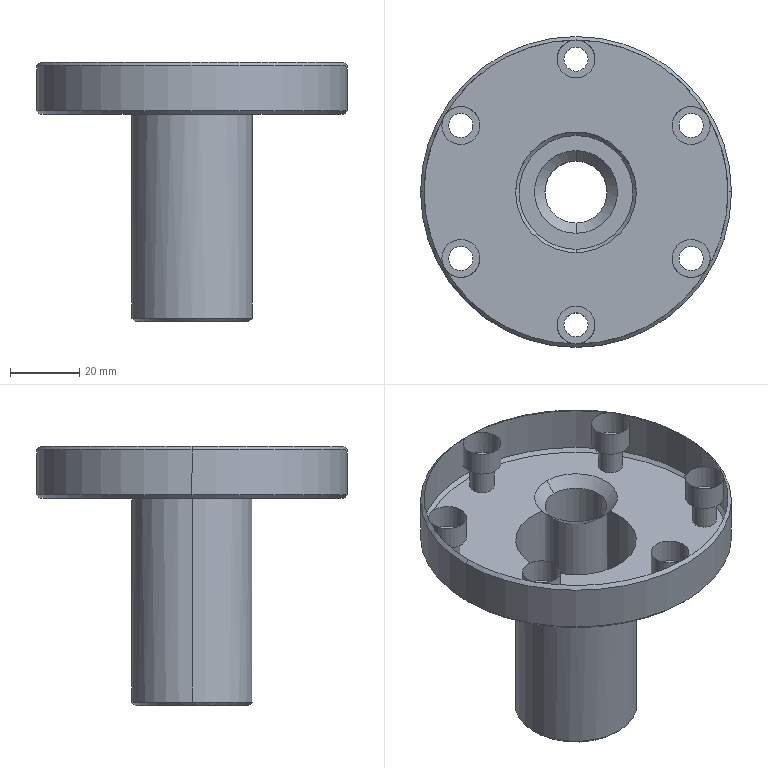Part | STEP file | Tail End Cover | 1 solid | 49 faces | box 90 x 90 x 75 mm | volume 127582 mm3 | cylinder 30 | cone 10 | plane 9 | commonest cylinder face diameters 7 x12 11 x12 18 x2 35 x2 90 x2
STEP:
#1=CARTESIAN_POINT('',(44.,0.,15.));
#2=VERTEX_POINT('',#1);
#3=CARTESIAN_POINT('',(0.,44.,15.));
#4=VERTEX_POINT('',#3);
#5=CARTESIAN_POINT('',(0.,0.,15.));
#6=DIRECTION('',(0.,0.,1.));
#7=DIRECTION('',(-1.,0.,0.));
#8=AXIS2_PLACEMENT_3D('',#5,#6,#7);
#9=CIRCLE('',#8,44.);
#10=EDGE_CURVE('',#2,#4,#9,.T.);
#11=ORIENTED_EDGE('',*,*,#10,.F.);
#12=CARTESIAN_POINT('',(45.,0.,14.));
#13=VERTEX_POINT('',#12);
#14=CARTESIAN_POINT('',(45.,0.,14.));
#15=DIRECTION('',(0.7071,0.,-0.7071));
#16=VECTOR('',#15,1000.);
#17=LINE('',#14,#16);
#18=EDGE_CURVE('',#2,#13,#17,.T.);
#19=ORIENTED_EDGE('',*,*,#18,.T.);
#20=CARTESIAN_POINT('',(-45.,0.,14.));
#21=VERTEX_POINT('',#20);
#22=CARTESIAN_POINT('',(0.,0.,14.));
#23=DIRECTION('',(0.,0.,1.));
#24=DIRECTION('',(-1.,0.,0.));
#25=AXIS2_PLACEMENT_3D('',#22,#23,#24);
#26=CIRCLE('',#25,45.);
#27=EDGE_CURVE('',#13,#21,#26,.T.);
#28=ORIENTED_EDGE('',*,*,#27,.T.);
#29=CARTESIAN_POINT('',(-44.,0.,15.));
#30=VERTEX_POINT('',#29);
#31=CARTESIAN_POINT('',(-45.,0.,14.));
#32=DIRECTION('',(-0.7071,0.,-0.7071));
#33=VECTOR('',#32,1000.);
#34=LINE('',#31,#33);
#35=EDGE_CURVE('',#30,#21,#34,.T.);
#36=ORIENTED_EDGE('',*,*,#35,.F.);
#37=CARTESIAN_POINT('',(-38.105,22.,15.));
#38=VERTEX_POINT('',#37);
#39=CARTESIAN_POINT('',(0.,0.,15.));
#40=DIRECTION('',(0.,0.,1.));
#41=DIRECTION('',(-1.,0.,0.));
#42=AXIS2_PLACEMENT_3D('',#39,#40,#41);
#43=CIRCLE('',#42,44.);
#44=EDGE_CURVE('',#38,#30,#43,.T.);
#45=ORIENTED_EDGE('',*,*,#44,.F.);
#46=CARTESIAN_POINT('',(0.,0.,15.));
#47=DIRECTION('',(0.,0.,1.));
#48=DIRECTION('',(-1.,0.,0.));
#49=AXIS2_PLACEMENT_3D('',#46,#47,#48);
#50=CIRCLE('',#49,44.);
#51=EDGE_CURVE('',#4,#38,#50,.T.);
#52=ORIENTED_EDGE('',*,*,#51,.F.);
#53=EDGE_LOOP('',(#11,#19,#28,#36,#45,#52));
#54=FACE_OUTER_BOUND('',#53,.T.);
#55=CARTESIAN_POINT('',(0.,0.,14.));
#56=DIRECTION('',(0.,0.,-1.));
#57=DIRECTION('',(-1.,0.,0.));
#58=AXIS2_PLACEMENT_3D('',#55,#56,#57);
#59=CONICAL_SURFACE('',#58,45.,0.7854);
#60=ADVANCED_FACE('',(#54),#59,.T.);
#61=CARTESIAN_POINT('',(27.842,-19.25,8.));
#62=VERTEX_POINT('',#61);
#63=CARTESIAN_POINT('',(38.842,-19.25,8.));
#64=VERTEX_POINT('',#63);
#65=CARTESIAN_POINT('',(33.342,-19.25,8.));
#66=DIRECTION('',(0.,0.,1.));
#67=DIRECTION('',(1.,0.,0.));
#68=AXIS2_PLACEMENT_3D('',#65,#66,#67);
#69=CIRCLE('',#68,5.5);
#70=EDGE_CURVE('',#62,#64,#69,.T.);
#71=ORIENTED_EDGE('',*,*,#70,.F.);
#72=CARTESIAN_POINT('',(27.842,-19.25,15.));
#73=VERTEX_POINT('',#72);
#74=CARTESIAN_POINT('',(27.842,-19.25,8.));
#75=DIRECTION('',(0.,0.,1.));
#76=VECTOR('',#75,1000.);
#77=LINE('',#74,#76);
#78=EDGE_CURVE('',#62,#73,#77,.T.);
#79=ORIENTED_EDGE('',*,*,#78,.T.);
#80=CARTESIAN_POINT('',(38.105,-22.,15.));
#81=VERTEX_POINT('',#80);
#82=CARTESIAN_POINT('',(33.342,-19.25,15.));
#83=DIRECTION('',(0.,0.,-1.));
#84=DIRECTION('',(1.,0.,0.));
#85=AXIS2_PLACEMENT_3D('',#82,#83,#84);
#86=CIRCLE('',#85,5.5);
#87=EDGE_CURVE('',#81,#73,#86,.T.);
#88=ORIENTED_EDGE('',*,*,#87,.F.);
#89=CARTESIAN_POINT('',(38.842,-19.25,15.));
#90=VERTEX_POINT('',#89);
#91=CARTESIAN_POINT('',(33.342,-19.25,15.));
#92=DIRECTION('',(0.,0.,-1.));
#93=DIRECTION('',(1.,0.,0.));
#94=AXIS2_PLACEMENT_3D('',#91,#92,#93);
#95=CIRCLE('',#94,5.5);
#96=EDGE_CURVE('',#90,#81,#95,.T.);
#97=ORIENTED_EDGE('',*,*,#96,.F.);
#98=CARTESIAN_POINT('',(38.842,-19.25,8.));
#99=DIRECTION('',(0.,0.,1.));
#100=VECTOR('',#99,1000.);
#101=LINE('',#98,#100);
#102=EDGE_CURVE('',#64,#90,#101,.T.);
#103=ORIENTED_EDGE('',*,*,#102,.F.);
#104=EDGE_LOOP('',(#71,#79,#88,#97,#103));
#105=FACE_OUTER_BOUND('',#104,.T.);
#106=CARTESIAN_POINT('',(33.342,-19.25,8.));
#107=DIRECTION('',(0.,0.,1.));
#108=DIRECTION('',(1.,0.,0.));
#109=AXIS2_PLACEMENT_3D('',#106,#107,#108);
#110=CYLINDRICAL_SURFACE('',#109,5.5);
#111=ADVANCED_FACE('',(#105),#110,.F.);
#112=CARTESIAN_POINT('',(-5.5,-38.5,8.));
#113=VERTEX_POINT('',#112);
#114=CARTESIAN_POINT('',(5.5,-38.5,8.));
#115=VERTEX_POINT('',#114);
#116=CARTESIAN_POINT('',(0.,-38.5,8.));
#117=DIRECTION('',(0.,0.,1.));
#118=DIRECTION('',(1.,0.,0.));
#119=AXIS2_PLACEMENT_3D('',#116,#117,#118);
#120=CIRCLE('',#119,5.5);
#121=EDGE_CURVE('',#113,#115,#120,.T.);
#122=ORIENTED_EDGE('',*,*,#121,.F.);
#123=CARTESIAN_POINT('',(-5.5,-38.5,15.));
#124=VERTEX_POINT('',#123);
#125=CARTESIAN_POINT('',(-5.5,-38.5,8.));
#126=DIRECTION('',(0.,0.,1.));
#127=VECTOR('',#126,1000.);
#128=LINE('',#125,#127);
#129=EDGE_CURVE('',#113,#124,#128,.T.);
#130=ORIENTED_EDGE('',*,*,#129,.T.);
#131=CARTESIAN_POINT('',(0.,-44.,15.));
#132=VERTEX_POINT('',#131);
#133=CARTESIAN_POINT('',(0.,-38.5,15.));
#134=DIRECTION('',(0.,0.,-1.));
#135=DIRECTION('',(1.,0.,0.));
#136=AXIS2_PLACEMENT_3D('',#133,#134,#135);
#137=CIRCLE('',#136,5.5);
#138=EDGE_CURVE('',#132,#124,#137,.T.);
#139=ORIENTED_EDGE('',*,*,#138,.F.);
#140=CARTESIAN_POINT('',(5.5,-38.5,15.));
#141=VERTEX_POINT('',#140);
#142=CARTESIAN_POINT('',(0.,-38.5,15.));
#143=DIRECTION('',(0.,0.,-1.));
#144=DIRECTION('',(1.,0.,0.));
#145=AXIS2_PLACEMENT_3D('',#142,#143,#144);
#146=CIRCLE('',#145,5.5);
#147=EDGE_CURVE('',#141,#132,#146,.T.);
#148=ORIENTED_EDGE('',*,*,#147,.F.);
#149=CARTESIAN_POINT('',(5.5,-38.5,8.));
#150=DIRECTION('',(0.,0.,1.));
#151=VECTOR('',#150,1000.);
#152=LINE('',#149,#151);
#153=EDGE_CURVE('',#115,#141,#152,.T.);
#154=ORIENTED_EDGE('',*,*,#153,.F.);
#155=EDGE_LOOP('',(#122,#130,#139,#148,#154));
#156=FACE_OUTER_BOUND('',#155,.T.);
#157=CARTESIAN_POINT('',(0.,-38.5,8.));
#158=DIRECTION('',(0.,0.,1.));
#159=DIRECTION('',(1.,0.,0.));
#160=AXIS2_PLACEMENT_3D('',#157,#158,#159);
#161=CYLINDRICAL_SURFACE('',#160,5.5);
#162=ADVANCED_FACE('',(#156),#161,.F.);
#163=CARTESIAN_POINT('',(-38.842,-19.25,8.));
#164=VERTEX_POINT('',#163);
#165=CARTESIAN_POINT('',(-27.842,-19.25,8.));
#166=VERTEX_POINT('',#165);
#167=CARTESIAN_POINT('',(-33.342,-19.25,8.));
#168=DIRECTION('',(0.,0.,1.));
#169=DIRECTION('',(1.,0.,0.));
#170=AXIS2_PLACEMENT_3D('',#167,#168,#169);
#171=CIRCLE('',#170,5.5);
#172=EDGE_CURVE('',#164,#166,#171,.T.);
#173=ORIENTED_EDGE('',*,*,#172,.F.);
#174=CARTESIAN_POINT('',(-38.842,-19.25,15.));
#175=VERTEX_POINT('',#174);
#176=CARTESIAN_POINT('',(-38.842,-19.25,8.));
#177=DIRECTION('',(0.,0.,1.));
#178=VECTOR('',#177,1000.);
#179=LINE('',#176,#178);
#180=EDGE_CURVE('',#164,#175,#179,.T.);
#181=ORIENTED_EDGE('',*,*,#180,.T.);
#182=CARTESIAN_POINT('',(-38.105,-22.,15.));
#183=VERTEX_POINT('',#182);
#184=CARTESIAN_POINT('',(-33.342,-19.25,15.));
#185=DIRECTION('',(0.,0.,-1.));
#186=DIRECTION('',(1.,0.,0.));
#187=AXIS2_PLACEMENT_3D('',#184,#185,#186);
#188=CIRCLE('',#187,5.5);
#189=EDGE_CURVE('',#183,#175,#188,.T.);
#190=ORIENTED_EDGE('',*,*,#189,.F.);
#191=CARTESIAN_POINT('',(-27.842,-19.25,15.));
#192=VERTEX_POINT('',#191);
#193=CARTESIAN_POINT('',(-33.342,-19.25,15.));
#194=DIRECTION('',(0.,0.,-1.));
#195=DIRECTION('',(1.,0.,0.));
#196=AXIS2_PLACEMENT_3D('',#193,#194,#195);
#197=CIRCLE('',#196,5.5);
#198=EDGE_CURVE('',#192,#183,#197,.T.);
#199=ORIENTED_EDGE('',*,*,#198,.F.);
#200=CARTESIAN_POINT('',(-27.842,-19.25,8.));
#201=DIRECTION('',(0.,0.,1.));
#202=VECTOR('',#201,1000.);
#203=LINE('',#200,#202);
#204=EDGE_CURVE('',#166,#192,#203,.T.);
#205=ORIENTED_EDGE('',*,*,#204,.F.);
#206=EDGE_LOOP('',(#173,#181,#190,#199,#205));
#207=FACE_OUTER_BOUND('',#206,.T.);
#208=CARTESIAN_POINT('',(-33.342,-19.25,8.));
#209=DIRECTION('',(0.,0.,1.));
#210=DIRECTION('',(1.,0.,0.));
#211=AXIS2_PLACEMENT_3D('',#208,#209,#210);
#212=CYLINDRICAL_SURFACE('',#211,5.5);
#213=ADVANCED_FACE('',(#207),#212,.F.);
#214=CARTESIAN_POINT('',(-38.842,19.25,8.));
#215=VERTEX_POINT('',#214);
#216=CARTESIAN_POINT('',(-27.842,19.25,8.));
#217=VERTEX_POINT('',#216);
#218=CARTESIAN_POINT('',(-33.342,19.25,8.));
#219=DIRECTION('',(0.,0.,1.));
#220=DIRECTION('',(1.,0.,0.));
#221=AXIS2_PLACEMENT_3D('',#218,#219,#220);
#222=CIRCLE('',#221,5.5);
#223=EDGE_CURVE('',#215,#217,#222,.T.);
#224=ORIENTED_EDGE('',*,*,#223,.F.);
#225=CARTESIAN_POINT('',(-38.842,19.25,15.));
#226=VERTEX_POINT('',#225);
#227=CARTESIAN_POINT('',(-38.842,19.25,8.));
#228=DIRECTION('',(0.,0.,1.));
#229=VECTOR('',#228,1000.);
#230=LINE('',#227,#229);
#231=EDGE_CURVE('',#215,#226,#230,.T.);
#232=ORIENTED_EDGE('',*,*,#231,.T.);
#233=CARTESIAN_POINT('',(-27.842,19.25,15.));
#234=VERTEX_POINT('',#233);
#235=CARTESIAN_POINT('',(-33.342,19.25,15.));
#236=DIRECTION('',(0.,0.,-1.));
#237=DIRECTION('',(1.,0.,0.));
#238=AXIS2_PLACEMENT_3D('',#235,#236,#237);
#239=CIRCLE('',#238,5.5);
#240=EDGE_CURVE('',#234,#226,#239,.T.);
#241=ORIENTED_EDGE('',*,*,#240,.F.);
#242=CARTESIAN_POINT('',(-27.842,19.25,8.));
#243=DIRECTION('',(0.,0.,1.));
#244=VECTOR('',#243,1000.);
#245=LINE('',#242,#244);
#246=EDGE_CURVE('',#217,#234,#245,.T.);
#247=ORIENTED_EDGE('',*,*,#246,.F.);
#248=EDGE_LOOP('',(#224,#232,#241,#247));
#249=FACE_OUTER_BOUND('',#248,.T.);
#250=CARTESIAN_POINT('',(-33.342,19.25,8.));
#251=DIRECTION('',(0.,0.,1.));
#252=DIRECTION('',(1.,0.,0.));
#253=AXIS2_PLACEMENT_3D('',#250,#251,#252);
#254=CYLINDRICAL_SURFACE('',#253,5.5);
#255=ADVANCED_FACE('',(#249),#254,.F.);
#256=CARTESIAN_POINT('',(-5.5,38.5,8.));
#257=VERTEX_POINT('',#256);
#258=CARTESIAN_POINT('',(5.5,38.5,8.));
#259=VERTEX_POINT('',#258);
#260=CARTESIAN_POINT('',(0.,38.5,8.));
#261=DIRECTION('',(0.,0.,1.));
#262=DIRECTION('',(1.,0.,0.));
#263=AXIS2_PLACEMENT_3D('',#260,#261,#262);
#264=CIRCLE('',#263,5.5);
#265=EDGE_CURVE('',#257,#259,#264,.T.);
#266=ORIENTED_EDGE('',*,*,#265,.F.);
#267=CARTESIAN_POINT('',(-5.5,38.5,15.));
#268=VERTEX_POINT('',#267);
#269=CARTESIAN_POINT('',(-5.5,38.5,8.));
#270=DIRECTION('',(0.,0.,1.));
#271=VECTOR('',#270,1000.);
#272=LINE('',#269,#271);
#273=EDGE_CURVE('',#257,#268,#272,.T.);
#274=ORIENTED_EDGE('',*,*,#273,.T.);
#275=CARTESIAN_POINT('',(5.5,38.5,15.));
#276=VERTEX_POINT('',#275);
#277=CARTESIAN_POINT('',(0.,38.5,15.));
#278=DIRECTION('',(0.,0.,-1.));
#279=DIRECTION('',(1.,0.,0.));
#280=AXIS2_PLACEMENT_3D('',#277,#278,#279);
#281=CIRCLE('',#280,5.5);
#282=EDGE_CURVE('',#276,#268,#281,.T.);
#283=ORIENTED_EDGE('',*,*,#282,.F.);
#284=CARTESIAN_POINT('',(5.5,38.5,8.));
#285=DIRECTION('',(0.,0.,1.));
#286=VECTOR('',#285,1000.);
#287=LINE('',#284,#286);
#288=EDGE_CURVE('',#259,#276,#287,.T.);
#289=ORIENTED_EDGE('',*,*,#288,.F.);
#290=EDGE_LOOP('',(#266,#274,#283,#289));
#291=FACE_OUTER_BOUND('',#290,.T.);
#292=CARTESIAN_POINT('',(0.,38.5,8.));
#293=DIRECTION('',(0.,0.,1.));
#294=DIRECTION('',(1.,0.,0.));
#295=AXIS2_PLACEMENT_3D('',#292,#293,#294);
#296=CYLINDRICAL_SURFACE('',#295,5.5);
#297=ADVANCED_FACE('',(#291),#296,.F.);
#298=CARTESIAN_POINT('',(27.842,19.25,8.));
#299=VERTEX_POINT('',#298);
#300=CARTESIAN_POINT('',(38.842,19.25,8.));
#301=VERTEX_POINT('',#300);
#302=CARTESIAN_POINT('',(33.342,19.25,8.));
#303=DIRECTION('',(0.,0.,1.));
#304=DIRECTION('',(1.,0.,0.));
#305=AXIS2_PLACEMENT_3D('',#302,#303,#304);
#306=CIRCLE('',#305,5.5);
#307=EDGE_CURVE('',#299,#301,#306,.T.);
#308=ORIENTED_EDGE('',*,*,#307,.F.);
#309=CARTESIAN_POINT('',(27.842,19.25,15.));
#310=VERTEX_POINT('',#309);
#311=CARTESIAN_POINT('',(27.842,19.25,8.));
#312=DIRECTION('',(0.,0.,1.));
#313=VECTOR('',#312,1000.);
#314=LINE('',#311,#313);
#315=EDGE_CURVE('',#299,#310,#314,.T.);
#316=ORIENTED_EDGE('',*,*,#315,.T.);
#317=CARTESIAN_POINT('',(38.842,19.25,15.));
#318=VERTEX_POINT('',#317);
#319=CARTESIAN_POINT('',(33.342,19.25,15.));
#320=DIRECTION('',(0.,0.,-1.));
#321=DIRECTION('',(1.,0.,0.));
#322=AXIS2_PLACEMENT_3D('',#319,#320,#321);
#323=CIRCLE('',#322,5.5);
#324=EDGE_CURVE('',#318,#310,#323,.T.);
#325=ORIENTED_EDGE('',*,*,#324,.F.);
#326=CARTESIAN_POINT('',(38.842,19.25,8.));
#327=DIRECTION('',(0.,0.,1.));
#328=VECTOR('',#327,1000.);
#329=LINE('',#326,#328);
#330=EDGE_CURVE('',#301,#318,#329,.T.);
#331=ORIENTED_EDGE('',*,*,#330,.F.);
#332=EDGE_LOOP('',(#308,#316,#325,#331));
#333=FACE_OUTER_BOUND('',#332,.T.);
#334=CARTESIAN_POINT('',(33.342,19.25,8.));
#335=DIRECTION('',(0.,0.,1.));
#336=DIRECTION('',(1.,0.,0.));
#337=AXIS2_PLACEMENT_3D('',#334,#335,#336);
#338=CYLINDRICAL_SURFACE('',#337,5.5);
#339=ADVANCED_FACE('',(#333),#338,.F.);
#340=CARTESIAN_POINT('',(0.,9.,12.));
#341=VERTEX_POINT('',#340);
#342=CARTESIAN_POINT('',(-9.,0.,12.));
#343=VERTEX_POINT('',#342);
#344=CARTESIAN_POINT('',(0.,0.,12.));
#345=DIRECTION('',(0.,0.,1.));
#346=DIRECTION('',(1.,0.,0.));
#347=AXIS2_PLACEMENT_3D('',#344,#345,#346);
#348=CIRCLE('',#347,9.);
#349=EDGE_CURVE('',#341,#343,#348,.T.);
#350=ORIENTED_EDGE('',*,*,#349,.F.);
#351=CARTESIAN_POINT('',(0.,12.,15.));
#352=VERTEX_POINT('',#351);
#353=CARTESIAN_POINT('',(0.,12.,15.));
#354=DIRECTION('',(0.,0.7071,0.7071));
#355=VECTOR('',#354,1000.);
#356=LINE('',#353,#355);
#357=EDGE_CURVE('',#341,#352,#356,.T.);
#358=ORIENTED_EDGE('',*,*,#357,.T.);
#359=CARTESIAN_POINT('',(0.,-12.,15.));
#360=VERTEX_POINT('',#359);
#361=CARTESIAN_POINT('',(0.,0.,15.));
#362=DIRECTION('',(0.,0.,-1.));
#363=DIRECTION('',(0.,-1.,0.));
#364=AXIS2_PLACEMENT_3D('',#361,#362,#363);
#365=CIRCLE('',#364,12.);
#366=EDGE_CURVE('',#360,#352,#365,.T.);
#367=ORIENTED_EDGE('',*,*,#366,.F.);
#368=CARTESIAN_POINT('',(0.,-9.,12.));
#369=VERTEX_POINT('',#368);
#370=CARTESIAN_POINT('',(0.,-12.,15.));
#371=DIRECTION('',(0.,-0.7071,0.7071));
#372=VECTOR('',#371,1000.);
#373=LINE('',#370,#372);
#374=EDGE_CURVE('',#369,#360,#373,.T.);
#375=ORIENTED_EDGE('',*,*,#374,.F.);
#376=CARTESIAN_POINT('',(0.,0.,12.));
#377=DIRECTION('',(0.,0.,1.));
#378=DIRECTION('',(1.,0.,0.));
#379=AXIS2_PLACEMENT_3D('',#376,#377,#378);
#380=CIRCLE('',#379,9.);
#381=EDGE_CURVE('',#343,#369,#380,.T.);
#382=ORIENTED_EDGE('',*,*,#381,.F.);
#383=EDGE_LOOP('',(#350,#358,#367,#375,#382));
#384=FACE_OUTER_BOUND('',#383,.T.);
#385=CARTESIAN_POINT('',(0.,0.,15.));
#386=DIRECTION('',(0.,0.,1.));
#387=DIRECTION('',(0.,-1.,0.));
#388=AXIS2_PLACEMENT_3D('',#385,#386,#387);
#389=CONICAL_SURFACE('',#388,12.,0.7854);
#390=ADVANCED_FACE('',(#384),#389,.F.);
#391=ORIENTED_EDGE('',*,*,#27,.F.);
#392=CARTESIAN_POINT('',(45.,0.,1.));
#393=VERTEX_POINT('',#392);
#394=CARTESIAN_POINT('',(45.,0.,15.));
#395=DIRECTION('',(0.,0.,-1.));
#396=VECTOR('',#395,1000.);
#397=LINE('',#394,#396);
#398=EDGE_CURVE('',#13,#393,#397,.T.);
#399=ORIENTED_EDGE('',*,*,#398,.T.);
#400=CARTESIAN_POINT('',(-45.,0.,1.));
#401=VERTEX_POINT('',#400);
#402=CARTESIAN_POINT('',(0.,0.,1.));
#403=DIRECTION('',(0.,0.,1.));
#404=DIRECTION('',(-1.,0.,0.));
#405=AXIS2_PLACEMENT_3D('',#402,#403,#404);
#406=CIRCLE('',#405,45.);
#407=EDGE_CURVE('',#393,#401,#406,.T.);
#408=ORIENTED_EDGE('',*,*,#407,.T.);
#409=CARTESIAN_POINT('',(-45.,0.,15.));
#410=DIRECTION('',(0.,0.,-1.));
#411=VECTOR('',#410,1000.);
#412=LINE('',#409,#411);
#413=EDGE_CURVE('',#21,#401,#412,.T.);
#414=ORIENTED_EDGE('',*,*,#413,.F.);
#415=EDGE_LOOP('',(#391,#399,#408,#414));
#416=FACE_OUTER_BOUND('',#415,.T.);
#417=CARTESIAN_POINT('',(0.,0.,15.));
#418=DIRECTION('',(0.,0.,-1.));
#419=DIRECTION('',(-1.,0.,0.));
#420=AXIS2_PLACEMENT_3D('',#417,#418,#419);
#421=CYLINDRICAL_SURFACE('',#420,45.);
#422=ADVANCED_FACE('',(#416),#421,.T.);
#423=ORIENTED_EDGE('',*,*,#381,.T.);
#424=CARTESIAN_POINT('',(9.,0.,12.));
#425=VERTEX_POINT('',#424);
#426=CARTESIAN_POINT('',(0.,0.,12.));
#427=DIRECTION('',(0.,0.,1.));
#428=DIRECTION('',(1.,0.,0.));
#429=AXIS2_PLACEMENT_3D('',#426,#427,#428);
#430=CIRCLE('',#429,9.);
#431=EDGE_CURVE('',#369,#425,#430,.T.);
#432=ORIENTED_EDGE('',*,*,#431,.T.);
#433=CARTESIAN_POINT('',(9.,0.,-59.));
#434=VERTEX_POINT('',#433);
#435=CARTESIAN_POINT('',(9.,0.,15.));
#436=DIRECTION('',(0.,0.,-1.));
#437=VECTOR('',#436,1000.);
#438=LINE('',#435,#437);
#439=EDGE_CURVE('',#425,#434,#438,.T.);
#440=ORIENTED_EDGE('',*,*,#439,.T.);
#441=CARTESIAN_POINT('',(0.,-9.,-59.));
#442=VERTEX_POINT('',#441);
#443=CARTESIAN_POINT('',(0.,0.,-59.));
#444=DIRECTION('',(0.,0.,1.));
#445=DIRECTION('',(-1.,0.,0.));
#446=AXIS2_PLACEMENT_3D('',#443,#444,#445);
#447=CIRCLE('',#446,9.);
#448=EDGE_CURVE('',#442,#434,#447,.T.);
#449=ORIENTED_EDGE('',*,*,#448,.F.);
#450=CARTESIAN_POINT('',(-9.,0.,-59.));
#451=VERTEX_POINT('',#450);
#452=CARTESIAN_POINT('',(0.,0.,-59.));
#453=DIRECTION('',(0.,0.,1.));
#454=DIRECTION('',(-1.,0.,0.));
#455=AXIS2_PLACEMENT_3D('',#452,#453,#454);
#456=CIRCLE('',#455,9.);
#457=EDGE_CURVE('',#451,#442,#456,.T.);
#458=ORIENTED_EDGE('',*,*,#457,.F.);
#459=CARTESIAN_POINT('',(-9.,0.,15.));
#460=DIRECTION('',(0.,0.,-1.));
#461=VECTOR('',#460,1000.);
#462=LINE('',#459,#461);
#463=EDGE_CURVE('',#343,#451,#462,.T.);
#464=ORIENTED_EDGE('',*,*,#463,.F.);
#465=EDGE_LOOP('',(#423,#432,#440,#449,#458,#464));
#466=FACE_OUTER_BOUND('',#465,.T.);
#467=CARTESIAN_POINT('',(0.,0.,15.));
#468=DIRECTION('',(0.,0.,-1.));
#469=DIRECTION('',(-1.,0.,0.));
#470=AXIS2_PLACEMENT_3D('',#467,#468,#469);
#471=CYLINDRICAL_SURFACE('',#470,9.);
#472=ADVANCED_FACE('',(#466),#471,.F.);
#473=CARTESIAN_POINT('',(44.,0.,0.));
#474=VERTEX_POINT('',#473);
#475=CARTESIAN_POINT('',(-44.,0.,0.));
#476=VERTEX_POINT('',#475);
#477=CARTESIAN_POINT('',(0.,0.,0.));
#478=DIRECTION('',(0.,0.,1.));
#479=DIRECTION('',(1.,0.,0.));
#480=AXIS2_PLACEMENT_3D('',#477,#478,#479);
#481=CIRCLE('',#480,44.);
#482=EDGE_CURVE('',#474,#476,#481,.T.);
#483=ORIENTED_EDGE('',*,*,#482,.T.);
#484=CARTESIAN_POINT('',(-45.,0.,1.));
#485=DIRECTION('',(-0.7071,0.,0.7071));
#486=VECTOR('',#485,1000.);
#487=LINE('',#484,#486);
#488=EDGE_CURVE('',#476,#401,#487,.T.);
#489=ORIENTED_EDGE('',*,*,#488,.T.);
#490=ORIENTED_EDGE('',*,*,#407,.F.);
#491=CARTESIAN_POINT('',(45.,0.,1.));
#492=DIRECTION('',(0.7071,0.,0.7071));
#493=VECTOR('',#492,1000.);
#494=LINE('',#491,#493);
#495=EDGE_CURVE('',#474,#393,#494,.T.);
#496=ORIENTED_EDGE('',*,*,#495,.F.);
#497=EDGE_LOOP('',(#483,#489,#490,#496));
#498=FACE_OUTER_BOUND('',#497,.T.);
#499=CARTESIAN_POINT('',(0.,0.,1.));
#500=DIRECTION('',(0.,0.,1.));
#501=DIRECTION('',(1.,0.,0.));
#502=AXIS2_PLACEMENT_3D('',#499,#500,#501);
#503=CONICAL_SURFACE('',#502,45.,0.7854);
#504=ADVANCED_FACE('',(#498),#503,.T.);
#505=CARTESIAN_POINT('',(36.842,-19.25,8.));
#506=VERTEX_POINT('',#505);
#507=CARTESIAN_POINT('',(29.842,-19.25,8.));
#508=VERTEX_POINT('',#507);
#509=CARTESIAN_POINT('',(33.342,-19.25,8.));
#510=DIRECTION('',(0.,0.,-1.));
#511=DIRECTION('',(-1.,0.,0.));
#512=AXIS2_PLACEMENT_3D('',#509,#510,#511);
#513=CIRCLE('',#512,3.5);
#514=EDGE_CURVE('',#506,#508,#513,.T.);
#515=ORIENTED_EDGE('',*,*,#514,.F.);
#516=CARTESIAN_POINT('',(36.842,-19.25,0.));
#517=VERTEX_POINT('',#516);
#518=CARTESIAN_POINT('',(36.842,-19.25,15.));
#519=DIRECTION('',(0.,0.,-1.));
#520=VECTOR('',#519,1000.);
#521=LINE('',#518,#520);
#522=EDGE_CURVE('',#506,#517,#521,.T.);
#523=ORIENTED_EDGE('',*,*,#522,.T.);
#524=CARTESIAN_POINT('',(29.842,-19.25,0.));
#525=VERTEX_POINT('',#524);
#526=CARTESIAN_POINT('',(33.342,-19.25,0.));
#527=DIRECTION('',(0.,0.,1.));
#528=DIRECTION('',(-1.,0.,0.));
#529=AXIS2_PLACEMENT_3D('',#526,#527,#528);
#530=CIRCLE('',#529,3.5);
#531=EDGE_CURVE('',#525,#517,#530,.T.);
#532=ORIENTED_EDGE('',*,*,#531,.F.);
#533=CARTESIAN_POINT('',(29.842,-19.25,15.));
#534=DIRECTION('',(0.,0.,-1.));
#535=VECTOR('',#534,1000.);
#536=LINE('',#533,#535);
#537=EDGE_CURVE('',#508,#525,#536,.T.);
#538=ORIENTED_EDGE('',*,*,#537,.F.);
#539=EDGE_LOOP('',(#515,#523,#532,#538));
#540=FACE_OUTER_BOUND('',#539,.T.);
#541=CARTESIAN_POINT('',(33.342,-19.25,15.));
#542=DIRECTION('',(0.,0.,-1.));
#543=DIRECTION('',(-1.,0.,0.));
#544=AXIS2_PLACEMENT_3D('',#541,#542,#543);
#545=CYLINDRICAL_SURFACE('',#544,3.5);
#546=ADVANCED_FACE('',(#540),#545,.F.);
#547=CARTESIAN_POINT('',(3.5,-38.5,8.));
#548=VERTEX_POINT('',#547);
#549=CARTESIAN_POINT('',(-3.5,-38.5,8.));
#550=VERTEX_POINT('',#549);
#551=CARTESIAN_POINT('',(0.,-38.5,8.));
#552=DIRECTION('',(0.,0.,-1.));
#553=DIRECTION('',(-1.,0.,0.));
#554=AXIS2_PLACEMENT_3D('',#551,#552,#553);
#555=CIRCLE('',#554,3.5);
#556=EDGE_CURVE('',#548,#550,#555,.T.);
#557=ORIENTED_EDGE('',*,*,#556,.F.);
#558=CARTESIAN_POINT('',(3.5,-38.5,0.));
#559=VERTEX_POINT('',#558);
#560=CARTESIAN_POINT('',(3.5,-38.5,15.));
#561=DIRECTION('',(0.,0.,-1.));
#562=VECTOR('',#561,1000.);
#563=LINE('',#560,#562);
#564=EDGE_CURVE('',#548,#559,#563,.T.);
#565=ORIENTED_EDGE('',*,*,#564,.T.);
#566=CARTESIAN_POINT('',(-3.5,-38.5,0.));
#567=VERTEX_POINT('',#566);
#568=CARTESIAN_POINT('',(0.,-38.5,0.));
#569=DIRECTION('',(0.,0.,1.));
#570=DIRECTION('',(-1.,0.,0.));
#571=AXIS2_PLACEMENT_3D('',#568,#569,#570);
#572=CIRCLE('',#571,3.5);
#573=EDGE_CURVE('',#567,#559,#572,.T.);
#574=ORIENTED_EDGE('',*,*,#573,.F.);
#575=CARTESIAN_POINT('',(-3.5,-38.5,15.));
#576=DIRECTION('',(0.,0.,-1.));
#577=VECTOR('',#576,1000.);
#578=LINE('',#575,#577);
#579=EDGE_CURVE('',#550,#567,#578,.T.);
#580=ORIENTED_EDGE('',*,*,#579,.F.);
#581=EDGE_LOOP('',(#557,#565,#574,#580));
#582=FACE_OUTER_BOUND('',#581,.T.);
#583=CARTESIAN_POINT('',(0.,-38.5,15.));
#584=DIRECTION('',(0.,0.,-1.));
#585=DIRECTION('',(-1.,0.,0.));
#586=AXIS2_PLACEMENT_3D('',#583,#584,#585);
#587=CYLINDRICAL_SURFACE('',#586,3.5);
#588=ADVANCED_FACE('',(#582),#587,.F.);
#589=CARTESIAN_POINT('',(-29.842,-19.25,8.));
#590=VERTEX_POINT('',#589);
#591=CARTESIAN_POINT('',(-36.842,-19.25,8.));
#592=VERTEX_POINT('',#591);
#593=CARTESIAN_POINT('',(-33.342,-19.25,8.));
#594=DIRECTION('',(0.,0.,-1.));
#595=DIRECTION('',(-1.,0.,0.));
#596=AXIS2_PLACEMENT_3D('',#593,#594,#595);
#597=CIRCLE('',#596,3.5);
#598=EDGE_CURVE('',#590,#592,#597,.T.);
#599=ORIENTED_EDGE('',*,*,#598,.F.);
#600=CARTESIAN_POINT('',(-29.842,-19.25,0.));
#601=VERTEX_POINT('',#600);
#602=CARTESIAN_POINT('',(-29.842,-19.25,15.));
#603=DIRECTION('',(0.,0.,-1.));
#604=VECTOR('',#603,1000.);
#605=LINE('',#602,#604);
#606=EDGE_CURVE('',#590,#601,#605,.T.);
#607=ORIENTED_EDGE('',*,*,#606,.T.);
#608=CARTESIAN_POINT('',(-36.842,-19.25,0.));
#609=VERTEX_POINT('',#608);
#610=CARTESIAN_POINT('',(-33.342,-19.25,0.));
#611=DIRECTION('',(0.,0.,1.));
#612=DIRECTION('',(-1.,0.,0.));
#613=AXIS2_PLACEMENT_3D('',#610,#611,#612);
#614=CIRCLE('',#613,3.5);
#615=EDGE_CURVE('',#609,#601,#614,.T.);
#616=ORIENTED_EDGE('',*,*,#615,.F.);
#617=CARTESIAN_POINT('',(-36.842,-19.25,15.));
#618=DIRECTION('',(0.,0.,-1.));
#619=VECTOR('',#618,1000.);
#620=LINE('',#617,#619);
#621=EDGE_CURVE('',#592,#609,#620,.T.);
#622=ORIENTED_EDGE('',*,*,#621,.F.);
#623=EDGE_LOOP('',(#599,#607,#616,#622));
#624=FACE_OUTER_BOUND('',#623,.T.);
#625=CARTESIAN_POINT('',(-33.342,-19.25,15.));
#626=DIRECTION('',(0.,0.,-1.));
#627=DIRECTION('',(-1.,0.,0.));
#628=AXIS2_PLACEMENT_3D('',#625,#626,#627);
#629=CYLINDRICAL_SURFACE('',#628,3.5);
#630=ADVANCED_FACE('',(#624),#629,.F.);
#631=CARTESIAN_POINT('',(-29.842,19.25,8.));
#632=VERTEX_POINT('',#631);
#633=CARTESIAN_POINT('',(-36.842,19.25,8.));
#634=VERTEX_POINT('',#633);
#635=CARTESIAN_POINT('',(-33.342,19.25,8.));
#636=DIRECTION('',(0.,0.,-1.));
#637=DIRECTION('',(-1.,0.,0.));
#638=AXIS2_PLACEMENT_3D('',#635,#636,#637);
#639=CIRCLE('',#638,3.5);
#640=EDGE_CURVE('',#632,#634,#639,.T.);
#641=ORIENTED_EDGE('',*,*,#640,.F.);
#642=CARTESIAN_POINT('',(-29.842,19.25,0.));
#643=VERTEX_POINT('',#642);
#644=CARTESIAN_POINT('',(-29.842,19.25,15.));
#645=DIRECTION('',(0.,0.,-1.));
#646=VECTOR('',#645,1000.);
#647=LINE('',#644,#646);
#648=EDGE_CURVE('',#632,#643,#647,.T.);
#649=ORIENTED_EDGE('',*,*,#648,.T.);
#650=CARTESIAN_POINT('',(-36.842,19.25,0.));
#651=VERTEX_POINT('',#650);
#652=CARTESIAN_POINT('',(-33.342,19.25,0.));
#653=DIRECTION('',(0.,0.,1.));
#654=DIRECTION('',(-1.,0.,0.));
#655=AXIS2_PLACEMENT_3D('',#652,#653,#654);
#656=CIRCLE('',#655,3.5);
#657=EDGE_CURVE('',#651,#643,#656,.T.);
#658=ORIENTED_EDGE('',*,*,#657,.F.);
#659=CARTESIAN_POINT('',(-36.842,19.25,15.));
#660=DIRECTION('',(0.,0.,-1.));
#661=VECTOR('',#660,1000.);
#662=LINE('',#659,#661);
#663=EDGE_CURVE('',#634,#651,#662,.T.);
#664=ORIENTED_EDGE('',*,*,#663,.F.);
#665=EDGE_LOOP('',(#641,#649,#658,#664));
#666=FACE_OUTER_BOUND('',#665,.T.);
#667=CARTESIAN_POINT('',(-33.342,19.25,15.));
#668=DIRECTION('',(0.,0.,-1.));
#669=DIRECTION('',(-1.,0.,0.));
#670=AXIS2_PLACEMENT_3D('',#667,#668,#669);
#671=CYLINDRICAL_SURFACE('',#670,3.5);
#672=ADVANCED_FACE('',(#666),#671,.F.);
#673=CARTESIAN_POINT('',(3.5,38.5,8.));
#674=VERTEX_POINT('',#673);
#675=CARTESIAN_POINT('',(-3.5,38.5,8.));
#676=VERTEX_POINT('',#675);
#677=CARTESIAN_POINT('',(0.,38.5,8.));
#678=DIRECTION('',(0.,0.,-1.));
#679=DIRECTION('',(-1.,0.,0.));
#680=AXIS2_PLACEMENT_3D('',#677,#678,#679);
#681=CIRCLE('',#680,3.5);
#682=EDGE_CURVE('',#674,#676,#681,.T.);
#683=ORIENTED_EDGE('',*,*,#682,.F.);
#684=CARTESIAN_POINT('',(3.5,38.5,0.));
#685=VERTEX_POINT('',#684);
#686=CARTESIAN_POINT('',(3.5,38.5,15.));
#687=DIRECTION('',(0.,0.,-1.));
#688=VECTOR('',#687,1000.);
#689=LINE('',#686,#688);
#690=EDGE_CURVE('',#674,#685,#689,.T.);
#691=ORIENTED_EDGE('',*,*,#690,.T.);
#692=CARTESIAN_POINT('',(-3.5,38.5,0.));
#693=VERTEX_POINT('',#692);
#694=CARTESIAN_POINT('',(0.,38.5,0.));
#695=DIRECTION('',(0.,0.,1.));
#696=DIRECTION('',(-1.,0.,0.));
#697=AXIS2_PLACEMENT_3D('',#694,#695,#696);
#698=CIRCLE('',#697,3.5);
#699=EDGE_CURVE('',#693,#685,#698,.T.);
#700=ORIENTED_EDGE('',*,*,#699,.F.);
#701=CARTESIAN_POINT('',(-3.5,38.5,15.));
#702=DIRECTION('',(0.,0.,-1.));
#703=VECTOR('',#702,1000.);
#704=LINE('',#701,#703);
#705=EDGE_CURVE('',#676,#693,#704,.T.);
#706=ORIENTED_EDGE('',*,*,#705,.F.);
#707=EDGE_LOOP('',(#683,#691,#700,#706));
#708=FACE_OUTER_BOUND('',#707,.T.);
#709=CARTESIAN_POINT('',(0.,38.5,15.));
#710=DIRECTION('',(0.,0.,-1.));
#711=DIRECTION('',(-1.,0.,0.));
#712=AXIS2_PLACEMENT_3D('',#709,#710,#711);
#713=CYLINDRICAL_SURFACE('',#712,3.5);
#714=ADVANCED_FACE('',(#708),#713,.F.);
#715=CARTESIAN_POINT('',(36.842,19.25,8.));
#716=VERTEX_POINT('',#715);
#717=CARTESIAN_POINT('',(29.842,19.25,8.));
#718=VERTEX_POINT('',#717);
#719=CARTESIAN_POINT('',(33.342,19.25,8.));
#720=DIRECTION('',(0.,0.,-1.));
#721=DIRECTION('',(-1.,0.,0.));
#722=AXIS2_PLACEMENT_3D('',#719,#720,#721);
#723=CIRCLE('',#722,3.5);
#724=EDGE_CURVE('',#716,#718,#723,.T.);
#725=ORIENTED_EDGE('',*,*,#724,.F.);
#726=CARTESIAN_POINT('',(36.842,19.25,0.));
#727=VERTEX_POINT('',#726);
#728=CARTESIAN_POINT('',(36.842,19.25,15.));
#729=DIRECTION('',(0.,0.,-1.));
#730=VECTOR('',#729,1000.);
#731=LINE('',#728,#730);
#732=EDGE_CURVE('',#716,#727,#731,.T.);
#733=ORIENTED_EDGE('',*,*,#732,.T.);
#734=CARTESIAN_POINT('',(29.842,19.25,0.));
#735=VERTEX_POINT('',#734);
#736=CARTESIAN_POINT('',(33.342,19.25,0.));
#737=DIRECTION('',(0.,0.,1.));
#738=DIRECTION('',(-1.,0.,0.));
#739=AXIS2_PLACEMENT_3D('',#736,#737,#738);
#740=CIRCLE('',#739,3.5);
#741=EDGE_CURVE('',#735,#727,#740,.T.);
#742=ORIENTED_EDGE('',*,*,#741,.F.);
#743=CARTESIAN_POINT('',(29.842,19.25,15.));
#744=DIRECTION('',(0.,0.,-1.));
#745=VECTOR('',#744,1000.);
#746=LINE('',#743,#745);
#747=EDGE_CURVE('',#718,#735,#746,.T.);
#748=ORIENTED_EDGE('',*,*,#747,.F.);
#749=EDGE_LOOP('',(#725,#733,#742,#748));
#750=FACE_OUTER_BOUND('',#749,.T.);
#751=CARTESIAN_POINT('',(33.342,19.25,15.));
#752=DIRECTION('',(0.,0.,-1.));
#753=DIRECTION('',(-1.,0.,0.));
#754=AXIS2_PLACEMENT_3D('',#751,#752,#753);
#755=CYLINDRICAL_SURFACE('',#754,3.5);
#756=ADVANCED_FACE('',(#750),#755,.F.);
#757=CARTESIAN_POINT('',(0.,9.,-59.));
#758=VERTEX_POINT('',#757);
#759=CARTESIAN_POINT('',(0.,0.,-59.));
#760=DIRECTION('',(0.,0.,1.));
#761=DIRECTION('',(-1.,0.,0.));
#762=AXIS2_PLACEMENT_3D('',#759,#760,#761);
#763=CIRCLE('',#762,9.);
#764=EDGE_CURVE('',#758,#451,#763,.T.);
#765=ORIENTED_EDGE('',*,*,#764,.T.);
#766=ORIENTED_EDGE('',*,*,#457,.T.);
#767=CARTESIAN_POINT('',(0.,-10.,-60.));
#768=VERTEX_POINT('',#767);
#769=CARTESIAN_POINT('',(0.,-10.,-60.));
#770=DIRECTION('',(0.,-0.7071,-0.7071));
#771=VECTOR('',#770,1000.);
#772=LINE('',#769,#771);
#773=EDGE_CURVE('',#442,#768,#772,.T.);
#774=ORIENTED_EDGE('',*,*,#773,.T.);
#775=CARTESIAN_POINT('',(0.,10.,-60.));
#776=VERTEX_POINT('',#775);
#777=CARTESIAN_POINT('',(0.,0.,-60.));
#778=DIRECTION('',(0.,0.,1.));
#779=DIRECTION('',(0.,1.,0.));
#780=AXIS2_PLACEMENT_3D('',#777,#778,#779);
#781=CIRCLE('',#780,10.);
#782=EDGE_CURVE('',#776,#768,#781,.T.);
#783=ORIENTED_EDGE('',*,*,#782,.F.);
#784=CARTESIAN_POINT('',(0.,10.,-60.));
#785=DIRECTION('',(0.,0.7071,-0.7071));
#786=VECTOR('',#785,1000.);
#787=LINE('',#784,#786);
#788=EDGE_CURVE('',#758,#776,#787,.T.);
#789=ORIENTED_EDGE('',*,*,#788,.F.);
#790=EDGE_LOOP('',(#765,#766,#774,#783,#789));
#791=FACE_OUTER_BOUND('',#790,.T.);
#792=CARTESIAN_POINT('',(0.,0.,-60.));
#793=DIRECTION('',(0.,0.,-1.));
#794=DIRECTION('',(0.,1.,0.));
#795=AXIS2_PLACEMENT_3D('',#792,#793,#794);
#796=CONICAL_SURFACE('',#795,10.,0.7854);
#797=ADVANCED_FACE('',(#791),#796,.F.);
#798=CARTESIAN_POINT('',(0.,17.5,-59.));
#799=VERTEX_POINT('',#798);
#800=CARTESIAN_POINT('',(-17.5,0.,-59.));
#801=VERTEX_POINT('',#800);
#802=CARTESIAN_POINT('',(0.,0.,-59.));
#803=DIRECTION('',(0.,0.,1.));
#804=DIRECTION('',(1.,0.,0.));
#805=AXIS2_PLACEMENT_3D('',#802,#803,#804);
#806=CIRCLE('',#805,17.5);
#807=EDGE_CURVE('',#799,#801,#806,.T.);
#808=ORIENTED_EDGE('',*,*,#807,.T.);
#809=CARTESIAN_POINT('',(-17.5,0.,0.));
#810=VERTEX_POINT('',#809);
#811=CARTESIAN_POINT('',(-17.5,0.,-60.));
#812=DIRECTION('',(0.,0.,1.));
#813=VECTOR('',#812,1000.);
#814=LINE('',#811,#813);
#815=EDGE_CURVE('',#801,#810,#814,.T.);
#816=ORIENTED_EDGE('',*,*,#815,.T.);
#817=CARTESIAN_POINT('',(17.5,0.,0.));
#818=VERTEX_POINT('',#817);
#819=CARTESIAN_POINT('',(0.,0.,0.));
#820=DIRECTION('',(0.,0.,-1.));
#821=DIRECTION('',(1.,0.,0.));
#822=AXIS2_PLACEMENT_3D('',#819,#820,#821);
#823=CIRCLE('',#822,17.5);
#824=EDGE_CURVE('',#810,#818,#823,.T.);
#825=ORIENTED_EDGE('',*,*,#824,.T.);
#826=CARTESIAN_POINT('',(17.5,0.,-59.));
#827=VERTEX_POINT('',#826);
#828=CARTESIAN_POINT('',(17.5,0.,-60.));
#829=DIRECTION('',(0.,0.,1.));
#830=VECTOR('',#829,1000.);
#831=LINE('',#828,#830);
#832=EDGE_CURVE('',#827,#818,#831,.T.);
#833=ORIENTED_EDGE('',*,*,#832,.F.);
#834=CARTESIAN_POINT('',(0.,0.,-59.));
#835=DIRECTION('',(0.,0.,1.));
#836=DIRECTION('',(1.,0.,0.));
#837=AXIS2_PLACEMENT_3D('',#834,#835,#836);
#838=CIRCLE('',#837,17.5);
#839=EDGE_CURVE('',#827,#799,#838,.T.);
#840=ORIENTED_EDGE('',*,*,#839,.T.);
#841=EDGE_LOOP('',(#808,#816,#825,#833,#840));
#842=FACE_OUTER_BOUND('',#841,.T.);
#843=CARTESIAN_POINT('',(0.,0.,-60.));
#844=DIRECTION('',(0.,0.,1.));
#845=DIRECTION('',(1.,0.,0.));
#846=AXIS2_PLACEMENT_3D('',#843,#844,#845);
#847=CYLINDRICAL_SURFACE('',#846,17.5);
#848=ADVANCED_FACE('',(#842),#847,.T.);
#849=CARTESIAN_POINT('',(0.,16.5,-60.));
#850=VERTEX_POINT('',#849);
#851=CARTESIAN_POINT('',(0.,-16.5,-60.));
#852=VERTEX_POINT('',#851);
#853=CARTESIAN_POINT('',(0.,0.,-60.));
#854=DIRECTION('',(0.,0.,-1.));
#855=DIRECTION('',(0.,-1.,0.));
#856=AXIS2_PLACEMENT_3D('',#853,#854,#855);
#857=CIRCLE('',#856,16.5);
#858=EDGE_CURVE('',#850,#852,#857,.T.);
#859=ORIENTED_EDGE('',*,*,#858,.F.);
#860=CARTESIAN_POINT('',(0.,17.5,-59.));
#861=DIRECTION('',(0.,0.7071,0.7071));
#862=VECTOR('',#861,1000.);
#863=LINE('',#860,#862);
#864=EDGE_CURVE('',#850,#799,#863,.T.);
#865=ORIENTED_EDGE('',*,*,#864,.T.);
#866=ORIENTED_EDGE('',*,*,#839,.F.);
#867=CARTESIAN_POINT('',(0.,-17.5,-59.));
#868=VERTEX_POINT('',#867);
#869=CARTESIAN_POINT('',(0.,0.,-59.));
#870=DIRECTION('',(0.,0.,1.));
#871=DIRECTION('',(1.,0.,0.));
#872=AXIS2_PLACEMENT_3D('',#869,#870,#871);
#873=CIRCLE('',#872,17.5);
#874=EDGE_CURVE('',#868,#827,#873,.T.);
#875=ORIENTED_EDGE('',*,*,#874,.F.);
#876=CARTESIAN_POINT('',(0.,-17.5,-59.));
#877=DIRECTION('',(0.,-0.7071,0.7071));
#878=VECTOR('',#877,1000.);
#879=LINE('',#876,#878);
#880=EDGE_CURVE('',#852,#868,#879,.T.);
#881=ORIENTED_EDGE('',*,*,#880,.F.);
#882=EDGE_LOOP('',(#859,#865,#866,#875,#881));
#883=FACE_OUTER_BOUND('',#882,.T.);
#884=CARTESIAN_POINT('',(0.,0.,-59.));
#885=DIRECTION('',(0.,0.,1.));
#886=DIRECTION('',(0.,-1.,0.));
#887=AXIS2_PLACEMENT_3D('',#884,#885,#886);
#888=CONICAL_SURFACE('',#887,17.5,0.7854);
#889=ADVANCED_FACE('',(#883),#888,.T.);
#890=ORIENTED_EDGE('',*,*,#87,.T.);
#891=CARTESIAN_POINT('',(33.342,-19.25,15.));
#892=DIRECTION('',(0.,0.,-1.));
#893=DIRECTION('',(1.,0.,0.));
#894=AXIS2_PLACEMENT_3D('',#891,#892,#893);
#895=CIRCLE('',#894,5.5);
#896=EDGE_CURVE('',#73,#90,#895,.T.);
#897=ORIENTED_EDGE('',*,*,#896,.T.);
#898=ORIENTED_EDGE('',*,*,#96,.T.);
#899=CARTESIAN_POINT('',(0.,0.,15.));
#900=DIRECTION('',(0.,0.,1.));
#901=DIRECTION('',(-1.,0.,0.));
#902=AXIS2_PLACEMENT_3D('',#899,#900,#901);
#903=CIRCLE('',#902,44.);
#904=EDGE_CURVE('',#81,#2,#903,.T.);
#905=ORIENTED_EDGE('',*,*,#904,.T.);
#906=ORIENTED_EDGE('',*,*,#10,.T.);
#907=CARTESIAN_POINT('',(0.,38.5,15.));
#908=DIRECTION('',(0.,0.,-1.));
#909=DIRECTION('',(1.,0.,0.));
#910=AXIS2_PLACEMENT_3D('',#907,#908,#909);
#911=CIRCLE('',#910,5.5);
#912=EDGE_CURVE('',#4,#276,#911,.T.);
#913=ORIENTED_EDGE('',*,*,#912,.T.);
#914=ORIENTED_EDGE('',*,*,#282,.T.);
#915=CARTESIAN_POINT('',(0.,38.5,15.));
#916=DIRECTION('',(0.,0.,-1.));
#917=DIRECTION('',(1.,0.,0.));
#918=AXIS2_PLACEMENT_3D('',#915,#916,#917);
#919=CIRCLE('',#918,5.5);
#920=EDGE_CURVE('',#268,#4,#919,.T.);
#921=ORIENTED_EDGE('',*,*,#920,.T.);
#922=ORIENTED_EDGE('',*,*,#51,.T.);
#923=CARTESIAN_POINT('',(-33.342,19.25,15.));
#924=DIRECTION('',(0.,0.,-1.));
#925=DIRECTION('',(1.,0.,0.));
#926=AXIS2_PLACEMENT_3D('',#923,#924,#925);
#927=CIRCLE('',#926,5.5);
#928=EDGE_CURVE('',#38,#234,#927,.T.);
#929=ORIENTED_EDGE('',*,*,#928,.T.);
#930=ORIENTED_EDGE('',*,*,#240,.T.);
#931=CARTESIAN_POINT('',(-33.342,19.25,15.));
#932=DIRECTION('',(0.,0.,-1.));
#933=DIRECTION('',(1.,0.,0.));
#934=AXIS2_PLACEMENT_3D('',#931,#932,#933);
#935=CIRCLE('',#934,5.5);
#936=EDGE_CURVE('',#226,#38,#935,.T.);
#937=ORIENTED_EDGE('',*,*,#936,.T.);
#938=ORIENTED_EDGE('',*,*,#44,.T.);
#939=CARTESIAN_POINT('',(0.,0.,15.));
#940=DIRECTION('',(0.,0.,1.));
#941=DIRECTION('',(-1.,0.,0.));
#942=AXIS2_PLACEMENT_3D('',#939,#940,#941);
#943=CIRCLE('',#942,44.);
#944=EDGE_CURVE('',#30,#183,#943,.T.);
#945=ORIENTED_EDGE('',*,*,#944,.T.);
#946=ORIENTED_EDGE('',*,*,#189,.T.);
#947=CARTESIAN_POINT('',(-33.342,-19.25,15.));
#948=DIRECTION('',(0.,0.,-1.));
#949=DIRECTION('',(1.,0.,0.));
#950=AXIS2_PLACEMENT_3D('',#947,#948,#949);
#951=CIRCLE('',#950,5.5);
#952=EDGE_CURVE('',#175,#192,#951,.T.);
#953=ORIENTED_EDGE('',*,*,#952,.T.);
#954=ORIENTED_EDGE('',*,*,#198,.T.);
#955=CARTESIAN_POINT('',(0.,0.,15.));
#956=DIRECTION('',(0.,0.,1.));
#957=DIRECTION('',(-1.,0.,0.));
#958=AXIS2_PLACEMENT_3D('',#955,#956,#957);
#959=CIRCLE('',#958,44.);
#960=EDGE_CURVE('',#183,#132,#959,.T.);
#961=ORIENTED_EDGE('',*,*,#960,.T.);
#962=ORIENTED_EDGE('',*,*,#138,.T.);
#963=CARTESIAN_POINT('',(0.,-38.5,15.));
#964=DIRECTION('',(0.,0.,-1.));
#965=DIRECTION('',(1.,0.,0.));
#966=AXIS2_PLACEMENT_3D('',#963,#964,#965);
#967=CIRCLE('',#966,5.5);
#968=EDGE_CURVE('',#124,#141,#967,.T.);
#969=ORIENTED_EDGE('',*,*,#968,.T.);
#970=ORIENTED_EDGE('',*,*,#147,.T.);
#971=CARTESIAN_POINT('',(0.,0.,15.));
#972=DIRECTION('',(0.,0.,1.));
#973=DIRECTION('',(-1.,0.,0.));
#974=AXIS2_PLACEMENT_3D('',#971,#972,#973);
#975=CIRCLE('',#974,44.);
#976=EDGE_CURVE('',#132,#81,#975,.T.);
#977=ORIENTED_EDGE('',*,*,#976,.T.);
#978=EDGE_LOOP('',(#890,#897,#898,#905,#906,#913,#914,#921,#922,#929,#930,#937,#938,#945,#946,#953,#954,#961,#962,#969,#970,#977));
#979=FACE_OUTER_BOUND('',#978,.T.);
#980=ORIENTED_EDGE('',*,*,#324,.T.);
#981=CARTESIAN_POINT('',(33.342,19.25,15.));
#982=DIRECTION('',(0.,0.,-1.));
#983=DIRECTION('',(1.,0.,0.));
#984=AXIS2_PLACEMENT_3D('',#981,#982,#983);
#985=CIRCLE('',#984,5.5);
#986=EDGE_CURVE('',#310,#318,#985,.T.);
#987=ORIENTED_EDGE('',*,*,#986,.T.);
#988=EDGE_LOOP('',(#980,#987));
#989=FACE_BOUND('',#988,.T.);
#990=ORIENTED_EDGE('',*,*,#366,.T.);
#991=CARTESIAN_POINT('',(0.,0.,15.));
#992=DIRECTION('',(0.,0.,-1.));
#993=DIRECTION('',(0.,-1.,0.));
#994=AXIS2_PLACEMENT_3D('',#991,#992,#993);
#995=CIRCLE('',#994,12.);
#996=EDGE_CURVE('',#352,#360,#995,.T.);
#997=ORIENTED_EDGE('',*,*,#996,.T.);
#998=EDGE_LOOP('',(#990,#997));
#999=FACE_BOUND('',#998,.T.);
#1000=CARTESIAN_POINT('',(0.,0.,15.));
#1001=DIRECTION('',(0.,0.,1.));
#1002=DIRECTION('',(1.,0.,0.));
#1003=AXIS2_PLACEMENT_3D('',#1000,#1001,#1002);
#1004=PLANE('',#1003);
#1005=ADVANCED_FACE('',(#979,#989,#999),#1004,.T.);
#1006=ORIENTED_EDGE('',*,*,#18,.F.);
#1007=ORIENTED_EDGE('',*,*,#904,.F.);
#1008=ORIENTED_EDGE('',*,*,#976,.F.);
#1009=ORIENTED_EDGE('',*,*,#960,.F.);
#1010=ORIENTED_EDGE('',*,*,#944,.F.);
#1011=ORIENTED_EDGE('',*,*,#35,.T.);
#1012=CARTESIAN_POINT('',(0.,0.,14.));
#1013=DIRECTION('',(0.,0.,1.));
#1014=DIRECTION('',(-1.,0.,0.));
#1015=AXIS2_PLACEMENT_3D('',#1012,#1013,#1014);
#1016=CIRCLE('',#1015,45.);
#1017=EDGE_CURVE('',#21,#13,#1016,.T.);
#1018=ORIENTED_EDGE('',*,*,#1017,.T.);
#1019=EDGE_LOOP('',(#1006,#1007,#1008,#1009,#1010,#1011,#1018));
#1020=FACE_OUTER_BOUND('',#1019,.T.);
#1021=CARTESIAN_POINT('',(0.,0.,14.));
#1022=DIRECTION('',(0.,0.,-1.));
#1023=DIRECTION('',(-1.,0.,0.));
#1024=AXIS2_PLACEMENT_3D('',#1021,#1022,#1023);
#1025=CONICAL_SURFACE('',#1024,45.,0.7854);
#1026=ADVANCED_FACE('',(#1020),#1025,.T.);
#1027=ORIENTED_EDGE('',*,*,#78,.F.);
#1028=CARTESIAN_POINT('',(33.342,-19.25,8.));
#1029=DIRECTION('',(0.,0.,1.));
#1030=DIRECTION('',(1.,0.,0.));
#1031=AXIS2_PLACEMENT_3D('',#1028,#1029,#1030);
#1032=CIRCLE('',#1031,5.5);
#1033=EDGE_CURVE('',#64,#62,#1032,.T.);
#1034=ORIENTED_EDGE('',*,*,#1033,.F.);
#1035=ORIENTED_EDGE('',*,*,#102,.T.);
#1036=ORIENTED_EDGE('',*,*,#896,.F.);
#1037=EDGE_LOOP('',(#1027,#1034,#1035,#1036));
#1038=FACE_OUTER_BOUND('',#1037,.T.);
#1039=CARTESIAN_POINT('',(33.342,-19.25,8.));
#1040=DIRECTION('',(0.,0.,1.));
#1041=DIRECTION('',(1.,0.,0.));
#1042=AXIS2_PLACEMENT_3D('',#1039,#1040,#1041);
#1043=CYLINDRICAL_SURFACE('',#1042,5.5);
#1044=ADVANCED_FACE('',(#1038),#1043,.F.);
#1045=ORIENTED_EDGE('',*,*,#129,.F.);
#1046=CARTESIAN_POINT('',(0.,-38.5,8.));
#1047=DIRECTION('',(0.,0.,1.));
#1048=DIRECTION('',(1.,0.,0.));
#1049=AXIS2_PLACEMENT_3D('',#1046,#1047,#1048);
#1050=CIRCLE('',#1049,5.5);
#1051=EDGE_CURVE('',#115,#113,#1050,.T.);
#1052=ORIENTED_EDGE('',*,*,#1051,.F.);
#1053=ORIENTED_EDGE('',*,*,#153,.T.);
#1054=ORIENTED_EDGE('',*,*,#968,.F.);
#1055=EDGE_LOOP('',(#1045,#1052,#1053,#1054));
#1056=FACE_OUTER_BOUND('',#1055,.T.);
#1057=CARTESIAN_POINT('',(0.,-38.5,8.));
#1058=DIRECTION('',(0.,0.,1.));
#1059=DIRECTION('',(1.,0.,0.));
#1060=AXIS2_PLACEMENT_3D('',#1057,#1058,#1059);
#1061=CYLINDRICAL_SURFACE('',#1060,5.5);
#1062=ADVANCED_FACE('',(#1056),#1061,.F.);
#1063=ORIENTED_EDGE('',*,*,#180,.F.);
#1064=CARTESIAN_POINT('',(-33.342,-19.25,8.));
#1065=DIRECTION('',(0.,0.,1.));
#1066=DIRECTION('',(1.,0.,0.));
#1067=AXIS2_PLACEMENT_3D('',#1064,#1065,#1066);
#1068=CIRCLE('',#1067,5.5);
#1069=EDGE_CURVE('',#166,#164,#1068,.T.);
#1070=ORIENTED_EDGE('',*,*,#1069,.F.);
#1071=ORIENTED_EDGE('',*,*,#204,.T.);
#1072=ORIENTED_EDGE('',*,*,#952,.F.);
#1073=EDGE_LOOP('',(#1063,#1070,#1071,#1072));
#1074=FACE_OUTER_BOUND('',#1073,.T.);
#1075=CARTESIAN_POINT('',(-33.342,-19.25,8.));
#1076=DIRECTION('',(0.,0.,1.));
#1077=DIRECTION('',(1.,0.,0.));
#1078=AXIS2_PLACEMENT_3D('',#1075,#1076,#1077);
#1079=CYLINDRICAL_SURFACE('',#1078,5.5);
#1080=ADVANCED_FACE('',(#1074),#1079,.F.);
#1081=ORIENTED_EDGE('',*,*,#231,.F.);
#1082=CARTESIAN_POINT('',(-33.342,19.25,8.));
#1083=DIRECTION('',(0.,0.,1.));
#1084=DIRECTION('',(1.,0.,0.));
#1085=AXIS2_PLACEMENT_3D('',#1082,#1083,#1084);
#1086=CIRCLE('',#1085,5.5);
#1087=EDGE_CURVE('',#217,#215,#1086,.T.);
#1088=ORIENTED_EDGE('',*,*,#1087,.F.);
#1089=ORIENTED_EDGE('',*,*,#246,.T.);
#1090=ORIENTED_EDGE('',*,*,#928,.F.);
#1091=ORIENTED_EDGE('',*,*,#936,.F.);
#1092=EDGE_LOOP('',(#1081,#1088,#1089,#1090,#1091));
#1093=FACE_OUTER_BOUND('',#1092,.T.);
#1094=CARTESIAN_POINT('',(-33.342,19.25,8.));
#1095=DIRECTION('',(0.,0.,1.));
#1096=DIRECTION('',(1.,0.,0.));
#1097=AXIS2_PLACEMENT_3D('',#1094,#1095,#1096);
#1098=CYLINDRICAL_SURFACE('',#1097,5.5);
#1099=ADVANCED_FACE('',(#1093),#1098,.F.);
#1100=ORIENTED_EDGE('',*,*,#273,.F.);
#1101=CARTESIAN_POINT('',(0.,38.5,8.));
#1102=DIRECTION('',(0.,0.,1.));
#1103=DIRECTION('',(1.,0.,0.));
#1104=AXIS2_PLACEMENT_3D('',#1101,#1102,#1103);
#1105=CIRCLE('',#1104,5.5);
#1106=EDGE_CURVE('',#259,#257,#1105,.T.);
#1107=ORIENTED_EDGE('',*,*,#1106,.F.);
#1108=ORIENTED_EDGE('',*,*,#288,.T.);
#1109=ORIENTED_EDGE('',*,*,#912,.F.);
#1110=ORIENTED_EDGE('',*,*,#920,.F.);
#1111=EDGE_LOOP('',(#1100,#1107,#1108,#1109,#1110));
#1112=FACE_OUTER_BOUND('',#1111,.T.);
#1113=CARTESIAN_POINT('',(0.,38.5,8.));
#1114=DIRECTION('',(0.,0.,1.));
#1115=DIRECTION('',(1.,0.,0.));
#1116=AXIS2_PLACEMENT_3D('',#1113,#1114,#1115);
#1117=CYLINDRICAL_SURFACE('',#1116,5.5);
#1118=ADVANCED_FACE('',(#1112),#1117,.F.);
#1119=ORIENTED_EDGE('',*,*,#315,.F.);
#1120=CARTESIAN_POINT('',(33.342,19.25,8.));
#1121=DIRECTION('',(0.,0.,1.));
#1122=DIRECTION('',(1.,0.,0.));
#1123=AXIS2_PLACEMENT_3D('',#1120,#1121,#1122);
#1124=CIRCLE('',#1123,5.5);
#1125=EDGE_CURVE('',#301,#299,#1124,.T.);
#1126=ORIENTED_EDGE('',*,*,#1125,.F.);
#1127=ORIENTED_EDGE('',*,*,#330,.T.);
#1128=ORIENTED_EDGE('',*,*,#986,.F.);
#1129=EDGE_LOOP('',(#1119,#1126,#1127,#1128));
#1130=FACE_OUTER_BOUND('',#1129,.T.);
#1131=CARTESIAN_POINT('',(33.342,19.25,8.));
#1132=DIRECTION('',(0.,0.,1.));
#1133=DIRECTION('',(1.,0.,0.));
#1134=AXIS2_PLACEMENT_3D('',#1131,#1132,#1133);
#1135=CYLINDRICAL_SURFACE('',#1134,5.5);
#1136=ADVANCED_FACE('',(#1130),#1135,.F.);
#1137=ORIENTED_EDGE('',*,*,#357,.F.);
#1138=CARTESIAN_POINT('',(0.,0.,12.));
#1139=DIRECTION('',(0.,0.,1.));
#1140=DIRECTION('',(1.,0.,0.));
#1141=AXIS2_PLACEMENT_3D('',#1138,#1139,#1140);
#1142=CIRCLE('',#1141,9.);
#1143=EDGE_CURVE('',#425,#341,#1142,.T.);
#1144=ORIENTED_EDGE('',*,*,#1143,.F.);
#1145=ORIENTED_EDGE('',*,*,#431,.F.);
#1146=ORIENTED_EDGE('',*,*,#374,.T.);
#1147=ORIENTED_EDGE('',*,*,#996,.F.);
#1148=EDGE_LOOP('',(#1137,#1144,#1145,#1146,#1147));
#1149=FACE_OUTER_BOUND('',#1148,.T.);
#1150=CARTESIAN_POINT('',(0.,0.,15.));
#1151=DIRECTION('',(0.,0.,1.));
#1152=DIRECTION('',(0.,-1.,0.));
#1153=AXIS2_PLACEMENT_3D('',#1150,#1151,#1152);
#1154=CONICAL_SURFACE('',#1153,12.,0.7854);
#1155=ADVANCED_FACE('',(#1149),#1154,.F.);
#1156=ORIENTED_EDGE('',*,*,#398,.F.);
#1157=ORIENTED_EDGE('',*,*,#1017,.F.);
#1158=ORIENTED_EDGE('',*,*,#413,.T.);
#1159=CARTESIAN_POINT('',(0.,0.,1.));
#1160=DIRECTION('',(0.,0.,1.));
#1161=DIRECTION('',(-1.,0.,0.));
#1162=AXIS2_PLACEMENT_3D('',#1159,#1160,#1161);
#1163=CIRCLE('',#1162,45.);
#1164=EDGE_CURVE('',#401,#393,#1163,.T.);
#1165=ORIENTED_EDGE('',*,*,#1164,.T.);
#1166=EDGE_LOOP('',(#1156,#1157,#1158,#1165));
#1167=FACE_OUTER_BOUND('',#1166,.T.);
#1168=CARTESIAN_POINT('',(0.,0.,15.));
#1169=DIRECTION('',(0.,0.,-1.));
#1170=DIRECTION('',(-1.,0.,0.));
#1171=AXIS2_PLACEMENT_3D('',#1168,#1169,#1170);
#1172=CYLINDRICAL_SURFACE('',#1171,45.);
#1173=ADVANCED_FACE('',(#1167),#1172,.T.);
#1174=ORIENTED_EDGE('',*,*,#1033,.T.);
#1175=ORIENTED_EDGE('',*,*,#70,.T.);
#1176=EDGE_LOOP('',(#1174,#1175));
#1177=FACE_OUTER_BOUND('',#1176,.T.);
#1178=CARTESIAN_POINT('',(33.342,-19.25,8.));
#1179=DIRECTION('',(0.,0.,-1.));
#1180=DIRECTION('',(-1.,0.,0.));
#1181=AXIS2_PLACEMENT_3D('',#1178,#1179,#1180);
#1182=CIRCLE('',#1181,3.5);
#1183=EDGE_CURVE('',#508,#506,#1182,.T.);
#1184=ORIENTED_EDGE('',*,*,#1183,.T.);
#1185=ORIENTED_EDGE('',*,*,#514,.T.);
#1186=EDGE_LOOP('',(#1184,#1185));
#1187=FACE_BOUND('',#1186,.T.);
#1188=CARTESIAN_POINT('',(33.342,-19.25,8.));
#1189=DIRECTION('',(0.,0.,1.));
#1190=DIRECTION('',(1.,0.,0.));
#1191=AXIS2_PLACEMENT_3D('',#1188,#1189,#1190);
#1192=PLANE('',#1191);
#1193=ADVANCED_FACE('',(#1177,#1187),#1192,.T.);
#1194=ORIENTED_EDGE('',*,*,#1051,.T.);
#1195=ORIENTED_EDGE('',*,*,#121,.T.);
#1196=EDGE_LOOP('',(#1194,#1195));
#1197=FACE_OUTER_BOUND('',#1196,.T.);
#1198=CARTESIAN_POINT('',(0.,-38.5,8.));
#1199=DIRECTION('',(0.,0.,-1.));
#1200=DIRECTION('',(-1.,0.,0.));
#1201=AXIS2_PLACEMENT_3D('',#1198,#1199,#1200);
#1202=CIRCLE('',#1201,3.5);
#1203=EDGE_CURVE('',#550,#548,#1202,.T.);
#1204=ORIENTED_EDGE('',*,*,#1203,.T.);
#1205=ORIENTED_EDGE('',*,*,#556,.T.);
#1206=EDGE_LOOP('',(#1204,#1205));
#1207=FACE_BOUND('',#1206,.T.);
#1208=CARTESIAN_POINT('',(0.,-38.5,8.));
#1209=DIRECTION('',(0.,0.,1.));
#1210=DIRECTION('',(1.,0.,0.));
#1211=AXIS2_PLACEMENT_3D('',#1208,#1209,#1210);
#1212=PLANE('',#1211);
#1213=ADVANCED_FACE('',(#1197,#1207),#1212,.T.);
#1214=ORIENTED_EDGE('',*,*,#1069,.T.);
#1215=ORIENTED_EDGE('',*,*,#172,.T.);
#1216=EDGE_LOOP('',(#1214,#1215));
#1217=FACE_OUTER_BOUND('',#1216,.T.);
#1218=CARTESIAN_POINT('',(-33.342,-19.25,8.));
#1219=DIRECTION('',(0.,0.,-1.));
#1220=DIRECTION('',(-1.,0.,0.));
#1221=AXIS2_PLACEMENT_3D('',#1218,#1219,#1220);
#1222=CIRCLE('',#1221,3.5);
#1223=EDGE_CURVE('',#592,#590,#1222,.T.);
#1224=ORIENTED_EDGE('',*,*,#1223,.T.);
#1225=ORIENTED_EDGE('',*,*,#598,.T.);
#1226=EDGE_LOOP('',(#1224,#1225));
#1227=FACE_BOUND('',#1226,.T.);
#1228=CARTESIAN_POINT('',(-33.342,-19.25,8.));
#1229=DIRECTION('',(0.,0.,1.));
#1230=DIRECTION('',(1.,0.,0.));
#1231=AXIS2_PLACEMENT_3D('',#1228,#1229,#1230);
#1232=PLANE('',#1231);
#1233=ADVANCED_FACE('',(#1217,#1227),#1232,.T.);
#1234=ORIENTED_EDGE('',*,*,#1087,.T.);
#1235=ORIENTED_EDGE('',*,*,#223,.T.);
#1236=EDGE_LOOP('',(#1234,#1235));
#1237=FACE_OUTER_BOUND('',#1236,.T.);
#1238=CARTESIAN_POINT('',(-33.342,19.25,8.));
#1239=DIRECTION('',(0.,0.,-1.));
#1240=DIRECTION('',(-1.,0.,0.));
#1241=AXIS2_PLACEMENT_3D('',#1238,#1239,#1240);
#1242=CIRCLE('',#1241,3.5);
#1243=EDGE_CURVE('',#634,#632,#1242,.T.);
#1244=ORIENTED_EDGE('',*,*,#1243,.T.);
#1245=ORIENTED_EDGE('',*,*,#640,.T.);
#1246=EDGE_LOOP('',(#1244,#1245));
#1247=FACE_BOUND('',#1246,.T.);
#1248=CARTESIAN_POINT('',(-33.342,19.25,8.));
#1249=DIRECTION('',(0.,0.,1.));
#1250=DIRECTION('',(1.,0.,0.));
#1251=AXIS2_PLACEMENT_3D('',#1248,#1249,#1250);
#1252=PLANE('',#1251);
#1253=ADVANCED_FACE('',(#1237,#1247),#1252,.T.);
#1254=ORIENTED_EDGE('',*,*,#1106,.T.);
#1255=ORIENTED_EDGE('',*,*,#265,.T.);
#1256=EDGE_LOOP('',(#1254,#1255));
#1257=FACE_OUTER_BOUND('',#1256,.T.);
#1258=CARTESIAN_POINT('',(0.,38.5,8.));
#1259=DIRECTION('',(0.,0.,-1.));
#1260=DIRECTION('',(-1.,0.,0.));
#1261=AXIS2_PLACEMENT_3D('',#1258,#1259,#1260);
#1262=CIRCLE('',#1261,3.5);
#1263=EDGE_CURVE('',#676,#674,#1262,.T.);
#1264=ORIENTED_EDGE('',*,*,#1263,.T.);
#1265=ORIENTED_EDGE('',*,*,#682,.T.);
#1266=EDGE_LOOP('',(#1264,#1265));
#1267=FACE_BOUND('',#1266,.T.);
#1268=CARTESIAN_POINT('',(0.,38.5,8.));
#1269=DIRECTION('',(0.,0.,1.));
#1270=DIRECTION('',(1.,0.,0.));
#1271=AXIS2_PLACEMENT_3D('',#1268,#1269,#1270);
#1272=PLANE('',#1271);
#1273=ADVANCED_FACE('',(#1257,#1267),#1272,.T.);
#1274=ORIENTED_EDGE('',*,*,#1125,.T.);
#1275=ORIENTED_EDGE('',*,*,#307,.T.);
#1276=EDGE_LOOP('',(#1274,#1275));
#1277=FACE_OUTER_BOUND('',#1276,.T.);
#1278=CARTESIAN_POINT('',(33.342,19.25,8.));
#1279=DIRECTION('',(0.,0.,-1.));
#1280=DIRECTION('',(-1.,0.,0.));
#1281=AXIS2_PLACEMENT_3D('',#1278,#1279,#1280);
#1282=CIRCLE('',#1281,3.5);
#1283=EDGE_CURVE('',#718,#716,#1282,.T.);
#1284=ORIENTED_EDGE('',*,*,#1283,.T.);
#1285=ORIENTED_EDGE('',*,*,#724,.T.);
#1286=EDGE_LOOP('',(#1284,#1285));
#1287=FACE_BOUND('',#1286,.T.);
#1288=CARTESIAN_POINT('',(33.342,19.25,8.));
#1289=DIRECTION('',(0.,0.,1.));
#1290=DIRECTION('',(1.,0.,0.));
#1291=AXIS2_PLACEMENT_3D('',#1288,#1289,#1290);
#1292=PLANE('',#1291);
#1293=ADVANCED_FACE('',(#1277,#1287),#1292,.T.);
#1294=ORIENTED_EDGE('',*,*,#439,.F.);
#1295=ORIENTED_EDGE('',*,*,#1143,.T.);
#1296=ORIENTED_EDGE('',*,*,#349,.T.);
#1297=ORIENTED_EDGE('',*,*,#463,.T.);
#1298=ORIENTED_EDGE('',*,*,#764,.F.);
#1299=CARTESIAN_POINT('',(0.,0.,-59.));
#1300=DIRECTION('',(0.,0.,1.));
#1301=DIRECTION('',(-1.,0.,0.));
#1302=AXIS2_PLACEMENT_3D('',#1299,#1300,#1301);
#1303=CIRCLE('',#1302,9.);
#1304=EDGE_CURVE('',#434,#758,#1303,.T.);
#1305=ORIENTED_EDGE('',*,*,#1304,.F.);
#1306=EDGE_LOOP('',(#1294,#1295,#1296,#1297,#1298,#1305));
#1307=FACE_OUTER_BOUND('',#1306,.T.);
#1308=CARTESIAN_POINT('',(0.,0.,15.));
#1309=DIRECTION('',(0.,0.,-1.));
#1310=DIRECTION('',(-1.,0.,0.));
#1311=AXIS2_PLACEMENT_3D('',#1308,#1309,#1310);
#1312=CYLINDRICAL_SURFACE('',#1311,9.);
#1313=ADVANCED_FACE('',(#1307),#1312,.F.);
#1314=ORIENTED_EDGE('',*,*,#488,.F.);
#1315=CARTESIAN_POINT('',(0.,0.,0.));
#1316=DIRECTION('',(0.,0.,1.));
#1317=DIRECTION('',(1.,0.,0.));
#1318=AXIS2_PLACEMENT_3D('',#1315,#1316,#1317);
#1319=CIRCLE('',#1318,44.);
#1320=EDGE_CURVE('',#476,#474,#1319,.T.);
#1321=ORIENTED_EDGE('',*,*,#1320,.T.);
#1322=ORIENTED_EDGE('',*,*,#495,.T.);
#1323=ORIENTED_EDGE('',*,*,#1164,.F.);
#1324=EDGE_LOOP('',(#1314,#1321,#1322,#1323));
#1325=FACE_OUTER_BOUND('',#1324,.T.);
#1326=CARTESIAN_POINT('',(0.,0.,1.));
#1327=DIRECTION('',(0.,0.,1.));
#1328=DIRECTION('',(1.,0.,0.));
#1329=AXIS2_PLACEMENT_3D('',#1326,#1327,#1328);
#1330=CONICAL_SURFACE('',#1329,45.,0.7854);
#1331=ADVANCED_FACE('',(#1325),#1330,.T.);
#1332=ORIENTED_EDGE('',*,*,#522,.F.);
#1333=ORIENTED_EDGE('',*,*,#1183,.F.);
#1334=ORIENTED_EDGE('',*,*,#537,.T.);
#1335=CARTESIAN_POINT('',(33.342,-19.25,0.));
#1336=DIRECTION('',(0.,0.,1.));
#1337=DIRECTION('',(-1.,0.,0.));
#1338=AXIS2_PLACEMENT_3D('',#1335,#1336,#1337);
#1339=CIRCLE('',#1338,3.5);
#1340=EDGE_CURVE('',#517,#525,#1339,.T.);
#1341=ORIENTED_EDGE('',*,*,#1340,.F.);
#1342=EDGE_LOOP('',(#1332,#1333,#1334,#1341));
#1343=FACE_OUTER_BOUND('',#1342,.T.);
#1344=CARTESIAN_POINT('',(33.342,-19.25,15.));
#1345=DIRECTION('',(0.,0.,-1.));
#1346=DIRECTION('',(-1.,0.,0.));
#1347=AXIS2_PLACEMENT_3D('',#1344,#1345,#1346);
#1348=CYLINDRICAL_SURFACE('',#1347,3.5);
#1349=ADVANCED_FACE('',(#1343),#1348,.F.);
#1350=ORIENTED_EDGE('',*,*,#564,.F.);
#1351=ORIENTED_EDGE('',*,*,#1203,.F.);
#1352=ORIENTED_EDGE('',*,*,#579,.T.);
#1353=CARTESIAN_POINT('',(0.,-38.5,0.));
#1354=DIRECTION('',(0.,0.,1.));
#1355=DIRECTION('',(-1.,0.,0.));
#1356=AXIS2_PLACEMENT_3D('',#1353,#1354,#1355);
#1357=CIRCLE('',#1356,3.5);
#1358=EDGE_CURVE('',#559,#567,#1357,.T.);
#1359=ORIENTED_EDGE('',*,*,#1358,.F.);
#1360=EDGE_LOOP('',(#1350,#1351,#1352,#1359));
#1361=FACE_OUTER_BOUND('',#1360,.T.);
#1362=CARTESIAN_POINT('',(0.,-38.5,15.));
#1363=DIRECTION('',(0.,0.,-1.));
#1364=DIRECTION('',(-1.,0.,0.));
#1365=AXIS2_PLACEMENT_3D('',#1362,#1363,#1364);
#1366=CYLINDRICAL_SURFACE('',#1365,3.5);
#1367=ADVANCED_FACE('',(#1361),#1366,.F.);
#1368=ORIENTED_EDGE('',*,*,#606,.F.);
#1369=ORIENTED_EDGE('',*,*,#1223,.F.);
#1370=ORIENTED_EDGE('',*,*,#621,.T.);
#1371=CARTESIAN_POINT('',(-33.342,-19.25,0.));
#1372=DIRECTION('',(0.,0.,1.));
#1373=DIRECTION('',(-1.,0.,0.));
#1374=AXIS2_PLACEMENT_3D('',#1371,#1372,#1373);
#1375=CIRCLE('',#1374,3.5);
#1376=EDGE_CURVE('',#601,#609,#1375,.T.);
#1377=ORIENTED_EDGE('',*,*,#1376,.F.);
#1378=EDGE_LOOP('',(#1368,#1369,#1370,#1377));
#1379=FACE_OUTER_BOUND('',#1378,.T.);
#1380=CARTESIAN_POINT('',(-33.342,-19.25,15.));
#1381=DIRECTION('',(0.,0.,-1.));
#1382=DIRECTION('',(-1.,0.,0.));
#1383=AXIS2_PLACEMENT_3D('',#1380,#1381,#1382);
#1384=CYLINDRICAL_SURFACE('',#1383,3.5);
#1385=ADVANCED_FACE('',(#1379),#1384,.F.);
#1386=ORIENTED_EDGE('',*,*,#648,.F.);
#1387=ORIENTED_EDGE('',*,*,#1243,.F.);
#1388=ORIENTED_EDGE('',*,*,#663,.T.);
#1389=CARTESIAN_POINT('',(-33.342,19.25,0.));
#1390=DIRECTION('',(0.,0.,1.));
#1391=DIRECTION('',(-1.,0.,0.));
#1392=AXIS2_PLACEMENT_3D('',#1389,#1390,#1391);
#1393=CIRCLE('',#1392,3.5);
#1394=EDGE_CURVE('',#643,#651,#1393,.T.);
#1395=ORIENTED_EDGE('',*,*,#1394,.F.);
#1396=EDGE_LOOP('',(#1386,#1387,#1388,#1395));
#1397=FACE_OUTER_BOUND('',#1396,.T.);
#1398=CARTESIAN_POINT('',(-33.342,19.25,15.));
#1399=DIRECTION('',(0.,0.,-1.));
#1400=DIRECTION('',(-1.,0.,0.));
#1401=AXIS2_PLACEMENT_3D('',#1398,#1399,#1400);
#1402=CYLINDRICAL_SURFACE('',#1401,3.5);
#1403=ADVANCED_FACE('',(#1397),#1402,.F.);
#1404=ORIENTED_EDGE('',*,*,#690,.F.);
#1405=ORIENTED_EDGE('',*,*,#1263,.F.);
#1406=ORIENTED_EDGE('',*,*,#705,.T.);
#1407=CARTESIAN_POINT('',(0.,38.5,0.));
#1408=DIRECTION('',(0.,0.,1.));
#1409=DIRECTION('',(-1.,0.,0.));
#1410=AXIS2_PLACEMENT_3D('',#1407,#1408,#1409);
#1411=CIRCLE('',#1410,3.5);
#1412=EDGE_CURVE('',#685,#693,#1411,.T.);
#1413=ORIENTED_EDGE('',*,*,#1412,.F.);
#1414=EDGE_LOOP('',(#1404,#1405,#1406,#1413));
#1415=FACE_OUTER_BOUND('',#1414,.T.);
#1416=CARTESIAN_POINT('',(0.,38.5,15.));
#1417=DIRECTION('',(0.,0.,-1.));
#1418=DIRECTION('',(-1.,0.,0.));
#1419=AXIS2_PLACEMENT_3D('',#1416,#1417,#1418);
#1420=CYLINDRICAL_SURFACE('',#1419,3.5);
#1421=ADVANCED_FACE('',(#1415),#1420,.F.);
#1422=ORIENTED_EDGE('',*,*,#732,.F.);
#1423=ORIENTED_EDGE('',*,*,#1283,.F.);
#1424=ORIENTED_EDGE('',*,*,#747,.T.);
#1425=CARTESIAN_POINT('',(33.342,19.25,0.));
#1426=DIRECTION('',(0.,0.,1.));
#1427=DIRECTION('',(-1.,0.,0.));
#1428=AXIS2_PLACEMENT_3D('',#1425,#1426,#1427);
#1429=CIRCLE('',#1428,3.5);
#1430=EDGE_CURVE('',#727,#735,#1429,.T.);
#1431=ORIENTED_EDGE('',*,*,#1430,.F.);
#1432=EDGE_LOOP('',(#1422,#1423,#1424,#1431));
#1433=FACE_OUTER_BOUND('',#1432,.T.);
#1434=CARTESIAN_POINT('',(33.342,19.25,15.));
#1435=DIRECTION('',(0.,0.,-1.));
#1436=DIRECTION('',(-1.,0.,0.));
#1437=AXIS2_PLACEMENT_3D('',#1434,#1435,#1436);
#1438=CYLINDRICAL_SURFACE('',#1437,3.5);
#1439=ADVANCED_FACE('',(#1433),#1438,.F.);
#1440=ORIENTED_EDGE('',*,*,#773,.F.);
#1441=ORIENTED_EDGE('',*,*,#448,.T.);
#1442=ORIENTED_EDGE('',*,*,#1304,.T.);
#1443=ORIENTED_EDGE('',*,*,#788,.T.);
#1444=CARTESIAN_POINT('',(0.,0.,-60.));
#1445=DIRECTION('',(0.,0.,1.));
#1446=DIRECTION('',(0.,1.,0.));
#1447=AXIS2_PLACEMENT_3D('',#1444,#1445,#1446);
#1448=CIRCLE('',#1447,10.);
#1449=EDGE_CURVE('',#768,#776,#1448,.T.);
#1450=ORIENTED_EDGE('',*,*,#1449,.F.);
#1451=EDGE_LOOP('',(#1440,#1441,#1442,#1443,#1450));
#1452=FACE_OUTER_BOUND('',#1451,.T.);
#1453=CARTESIAN_POINT('',(0.,0.,-60.));
#1454=DIRECTION('',(0.,0.,-1.));
#1455=DIRECTION('',(0.,1.,0.));
#1456=AXIS2_PLACEMENT_3D('',#1453,#1454,#1455);
#1457=CONICAL_SURFACE('',#1456,10.,0.7854);
#1458=ADVANCED_FACE('',(#1452),#1457,.F.);
#1459=CARTESIAN_POINT('',(0.,0.,0.));
#1460=DIRECTION('',(0.,0.,-1.));
#1461=DIRECTION('',(1.,0.,0.));
#1462=AXIS2_PLACEMENT_3D('',#1459,#1460,#1461);
#1463=CIRCLE('',#1462,17.5);
#1464=EDGE_CURVE('',#818,#810,#1463,.T.);
#1465=ORIENTED_EDGE('',*,*,#1464,.F.);
#1466=ORIENTED_EDGE('',*,*,#824,.F.);
#1467=EDGE_LOOP('',(#1465,#1466));
#1468=FACE_BOUND('',#1467,.T.);
#1469=ORIENTED_EDGE('',*,*,#615,.T.);
#1470=ORIENTED_EDGE('',*,*,#1376,.T.);
#1471=EDGE_LOOP('',(#1469,#1470));
#1472=FACE_BOUND('',#1471,.T.);
#1473=ORIENTED_EDGE('',*,*,#531,.T.);
#1474=ORIENTED_EDGE('',*,*,#1340,.T.);
#1475=EDGE_LOOP('',(#1473,#1474));
#1476=FACE_BOUND('',#1475,.T.);
#1477=ORIENTED_EDGE('',*,*,#699,.T.);
#1478=ORIENTED_EDGE('',*,*,#1412,.T.);
#1479=EDGE_LOOP('',(#1477,#1478));
#1480=FACE_BOUND('',#1479,.T.);
#1481=ORIENTED_EDGE('',*,*,#741,.T.);
#1482=ORIENTED_EDGE('',*,*,#1430,.T.);
#1483=EDGE_LOOP('',(#1481,#1482));
#1484=FACE_BOUND('',#1483,.T.);
#1485=ORIENTED_EDGE('',*,*,#573,.T.);
#1486=ORIENTED_EDGE('',*,*,#1358,.T.);
#1487=EDGE_LOOP('',(#1485,#1486));
#1488=FACE_BOUND('',#1487,.T.);
#1489=ORIENTED_EDGE('',*,*,#657,.T.);
#1490=ORIENTED_EDGE('',*,*,#1394,.T.);
#1491=EDGE_LOOP('',(#1489,#1490));
#1492=FACE_BOUND('',#1491,.T.);
#1493=ORIENTED_EDGE('',*,*,#482,.F.);
#1494=ORIENTED_EDGE('',*,*,#1320,.F.);
#1495=EDGE_LOOP('',(#1493,#1494));
#1496=FACE_OUTER_BOUND('',#1495,.T.);
#1497=CARTESIAN_POINT('',(0.,0.,0.));
#1498=DIRECTION('',(0.,0.,1.));
#1499=DIRECTION('',(1.,0.,0.));
#1500=AXIS2_PLACEMENT_3D('',#1497,#1498,#1499);
#1501=PLANE('',#1500);
#1502=ADVANCED_FACE('',(#1468,#1472,#1476,#1480,#1484,#1488,#1492,#1496),#1501,.F.);
#1503=CARTESIAN_POINT('',(0.,0.,-60.));
#1504=DIRECTION('',(0.,0.,-1.));
#1505=DIRECTION('',(0.,-1.,0.));
#1506=AXIS2_PLACEMENT_3D('',#1503,#1504,#1505);
#1507=CIRCLE('',#1506,16.5);
#1508=EDGE_CURVE('',#852,#850,#1507,.T.);
#1509=ORIENTED_EDGE('',*,*,#1508,.T.);
#1510=ORIENTED_EDGE('',*,*,#858,.T.);
#1511=EDGE_LOOP('',(#1509,#1510));
#1512=FACE_OUTER_BOUND('',#1511,.T.);
#1513=ORIENTED_EDGE('',*,*,#782,.T.);
#1514=ORIENTED_EDGE('',*,*,#1449,.T.);
#1515=EDGE_LOOP('',(#1513,#1514));
#1516=FACE_BOUND('',#1515,.T.);
#1517=CARTESIAN_POINT('',(0.,0.,-60.));
#1518=DIRECTION('',(0.,0.,-1.));
#1519=DIRECTION('',(-1.,0.,0.));
#1520=AXIS2_PLACEMENT_3D('',#1517,#1518,#1519);
#1521=PLANE('',#1520);
#1522=ADVANCED_FACE('',(#1512,#1516),#1521,.T.);
#1523=ORIENTED_EDGE('',*,*,#815,.F.);
#1524=CARTESIAN_POINT('',(0.,0.,-59.));
#1525=DIRECTION('',(0.,0.,1.));
#1526=DIRECTION('',(1.,0.,0.));
#1527=AXIS2_PLACEMENT_3D('',#1524,#1525,#1526);
#1528=CIRCLE('',#1527,17.5);
#1529=EDGE_CURVE('',#801,#868,#1528,.T.);
#1530=ORIENTED_EDGE('',*,*,#1529,.T.);
#1531=ORIENTED_EDGE('',*,*,#874,.T.);
#1532=ORIENTED_EDGE('',*,*,#832,.T.);
#1533=ORIENTED_EDGE('',*,*,#1464,.T.);
#1534=EDGE_LOOP('',(#1523,#1530,#1531,#1532,#1533));
#1535=FACE_OUTER_BOUND('',#1534,.T.);
#1536=CARTESIAN_POINT('',(0.,0.,-60.));
#1537=DIRECTION('',(0.,0.,1.));
#1538=DIRECTION('',(1.,0.,0.));
#1539=AXIS2_PLACEMENT_3D('',#1536,#1537,#1538);
#1540=CYLINDRICAL_SURFACE('',#1539,17.5);
#1541=ADVANCED_FACE('',(#1535),#1540,.T.);
#1542=ORIENTED_EDGE('',*,*,#864,.F.);
#1543=ORIENTED_EDGE('',*,*,#1508,.F.);
#1544=ORIENTED_EDGE('',*,*,#880,.T.);
#1545=ORIENTED_EDGE('',*,*,#1529,.F.);
#1546=ORIENTED_EDGE('',*,*,#807,.F.);
#1547=EDGE_LOOP('',(#1542,#1543,#1544,#1545,#1546));
#1548=FACE_OUTER_BOUND('',#1547,.T.);
#1549=CARTESIAN_POINT('',(0.,0.,-59.));
#1550=DIRECTION('',(0.,0.,1.));
#1551=DIRECTION('',(0.,-1.,0.));
#1552=AXIS2_PLACEMENT_3D('',#1549,#1550,#1551);
#1553=CONICAL_SURFACE('',#1552,17.5,0.7854);
#1554=ADVANCED_FACE('',(#1548),#1553,.T.);
#1555=CLOSED_SHELL('',(#60,#111,#162,#213,#255,#297,#339,#390,#422,#472,#504,#546,#588,#630,#672,#714,#756,#797,#848,#889,#1005,#1026,#1044,#1062,#1080,#1099,#1118,#1136,#1155,#1173,#1193,#1213,#1233,#1253,#1273,#1293,#1313,#1331,#1349,#1367,#1385,#1403,#1421,#1439,#1458,#1502,#1522,#1541,#1554));
#1556=MANIFOLD_SOLID_BREP('',#1555);
#1557=CARTESIAN_POINT('',(0.,0.,0.));
#1558=DIRECTION('',(0.,0.,1.));
#1559=DIRECTION('',(1.,0.,0.));
#1560=AXIS2_PLACEMENT_3D('',#1557,#1558,#1559);
#1561=(LENGTH_UNIT()NAMED_UNIT(*)SI_UNIT(.MILLI.,.METRE.));
#1562=UNCERTAINTY_MEASURE_WITH_UNIT(LENGTH_MEASURE(0.00001),#1561,'','');
#1563=(NAMED_UNIT(*)PLANE_ANGLE_UNIT()SI_UNIT($,.RADIAN.));
#1564=(NAMED_UNIT(*)SI_UNIT($,.STERADIAN.)SOLID_ANGLE_UNIT());
#1565=(GEOMETRIC_REPRESENTATION_CONTEXT(3)GLOBAL_UNCERTAINTY_ASSIGNED_CONTEXT((#1562))GLOBAL_UNIT_ASSIGNED_CONTEXT((#1561,#1563,#1564))REPRESENTATION_CONTEXT('',''));
#1566=ADVANCED_BREP_SHAPE_REPRESENTATION('',(#1556,#1560),#1565);